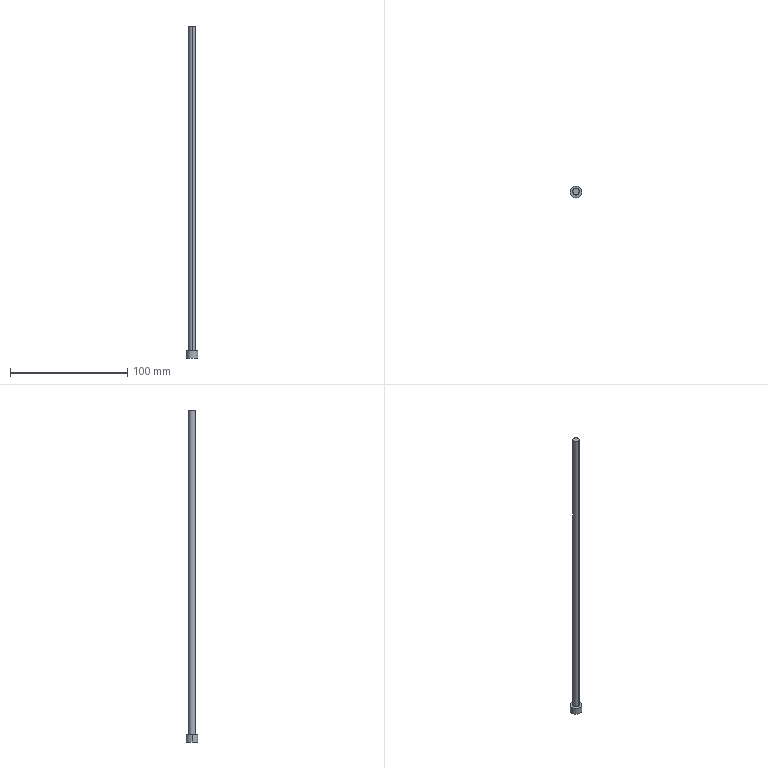Part | Creo | 1 solid | 7 faces | box 10 x 10 x 283.312 mm | volume 7060 mm3 | cylinder 4 | plane 3 | commonest cylinder face diameters 5.5 x2 10 x2
STEP:
#1=CARTESIAN_POINT('',(28.75,-153.,-12.688));
#2=VERTEX_POINT('',#1);
#3=CARTESIAN_POINT('',(26.,-150.25,-12.688));
#4=VERTEX_POINT('',#3);
#5=CARTESIAN_POINT('',(26.,-153.,-12.688));
#6=DIRECTION('',(0.,0.,1.));
#7=DIRECTION('',(1.,0.,0.));
#8=AXIS2_PLACEMENT_3D('',#5,#6,#7);
#9=CIRCLE('',#8,2.75);
#10=EDGE_CURVE('',#2,#4,#9,.T.);
#11=ORIENTED_EDGE('',*,*,#10,.F.);
#12=CARTESIAN_POINT('',(26.,-155.75,-12.688));
#13=VERTEX_POINT('',#12);
#14=CARTESIAN_POINT('',(26.,-153.,-12.688));
#15=DIRECTION('',(0.,0.,1.));
#16=DIRECTION('',(0.,-1.,0.));
#17=AXIS2_PLACEMENT_3D('',#14,#15,#16);
#18=CIRCLE('',#17,2.75);
#19=EDGE_CURVE('',#13,#2,#18,.T.);
#20=ORIENTED_EDGE('',*,*,#19,.F.);
#21=CARTESIAN_POINT('',(23.25,-153.,-12.688));
#22=VERTEX_POINT('',#21);
#23=CARTESIAN_POINT('',(26.,-153.,-12.688));
#24=DIRECTION('',(0.,0.,1.));
#25=DIRECTION('',(-1.,0.,0.));
#26=AXIS2_PLACEMENT_3D('',#23,#24,#25);
#27=CIRCLE('',#26,2.75);
#28=EDGE_CURVE('',#22,#13,#27,.T.);
#29=ORIENTED_EDGE('',*,*,#28,.F.);
#30=CARTESIAN_POINT('',(26.,-153.,-12.688));
#31=DIRECTION('',(0.,0.,1.));
#32=DIRECTION('',(0.,1.,0.));
#33=AXIS2_PLACEMENT_3D('',#30,#31,#32);
#34=CIRCLE('',#33,2.75);
#35=EDGE_CURVE('',#4,#22,#34,.T.);
#36=ORIENTED_EDGE('',*,*,#35,.F.);
#37=EDGE_LOOP('',(#11,#20,#29,#36));
#38=FACE_OUTER_BOUND('',#37,.F.);
#39=CARTESIAN_POINT('',(-2.3,-2.15,-12.688));
#40=DIRECTION('',(0.,0.,1.));
#41=DIRECTION('',(0.,-1.,0.));
#42=AXIS2_PLACEMENT_3D('',#39,#40,#41);
#43=PLANE('',#42);
#44=ADVANCED_FACE('',(#38),#43,.T.);
#45=CARTESIAN_POINT('',(26.,-150.25,-290.));
#46=VERTEX_POINT('',#45);
#47=CARTESIAN_POINT('',(28.75,-153.,-290.));
#48=VERTEX_POINT('',#47);
#49=CARTESIAN_POINT('',(26.,-153.,-290.));
#50=DIRECTION('',(0.,0.,-1.));
#51=DIRECTION('',(0.,1.,0.));
#52=AXIS2_PLACEMENT_3D('',#49,#50,#51);
#53=CIRCLE('',#52,2.75);
#54=EDGE_CURVE('',#46,#48,#53,.T.);
#55=ORIENTED_EDGE('',*,*,#54,.T.);
#56=CARTESIAN_POINT('',(26.,-155.75,-290.));
#57=VERTEX_POINT('',#56);
#58=CARTESIAN_POINT('',(26.,-153.,-290.));
#59=DIRECTION('',(0.,0.,-1.));
#60=DIRECTION('',(1.,0.,0.));
#61=AXIS2_PLACEMENT_3D('',#58,#59,#60);
#62=CIRCLE('',#61,2.75);
#63=EDGE_CURVE('',#48,#57,#62,.T.);
#64=ORIENTED_EDGE('',*,*,#63,.T.);
#65=CARTESIAN_POINT('',(26.,-155.75,-290.));
#66=DIRECTION('',(0.,0.,1.));
#67=VECTOR('',#66,277.312);
#68=LINE('',#65,#67);
#69=EDGE_CURVE('',#57,#13,#68,.T.);
#70=ORIENTED_EDGE('',*,*,#69,.T.);
#71=ORIENTED_EDGE('',*,*,#19,.T.);
#72=ORIENTED_EDGE('',*,*,#10,.T.);
#73=CARTESIAN_POINT('',(26.,-150.25,-290.));
#74=DIRECTION('',(0.,0.,1.));
#75=VECTOR('',#74,277.312);
#76=LINE('',#73,#75);
#77=EDGE_CURVE('',#46,#4,#76,.T.);
#78=ORIENTED_EDGE('',*,*,#77,.F.);
#79=EDGE_LOOP('',(#55,#64,#70,#71,#72,#78));
#80=FACE_OUTER_BOUND('',#79,.F.);
#81=CARTESIAN_POINT('',(26.,-153.,-351.57));
#82=DIRECTION('',(0.,0.,1.));
#83=DIRECTION('',(0.,-1.,0.));
#84=AXIS2_PLACEMENT_3D('',#81,#82,#83);
#85=CYLINDRICAL_SURFACE('',#84,2.75);
#86=ADVANCED_FACE('',(#80),#85,.T.);
#87=CARTESIAN_POINT('',(31.,-153.,-290.));
#88=VERTEX_POINT('',#87);
#89=CARTESIAN_POINT('',(21.,-153.,-290.));
#90=VERTEX_POINT('',#89);
#91=CARTESIAN_POINT('',(26.,-153.,-290.));
#92=DIRECTION('',(0.,0.,1.));
#93=DIRECTION('',(1.,0.,0.));
#94=AXIS2_PLACEMENT_3D('',#91,#92,#93);
#95=CIRCLE('',#94,5.);
#96=EDGE_CURVE('',#88,#90,#95,.T.);
#97=ORIENTED_EDGE('',*,*,#96,.F.);
#98=CARTESIAN_POINT('',(26.,-153.,-290.));
#99=DIRECTION('',(0.,0.,1.));
#100=DIRECTION('',(-1.,0.,0.));
#101=AXIS2_PLACEMENT_3D('',#98,#99,#100);
#102=CIRCLE('',#101,5.);
#103=EDGE_CURVE('',#90,#88,#102,.T.);
#104=ORIENTED_EDGE('',*,*,#103,.F.);
#105=EDGE_LOOP('',(#97,#104));
#106=FACE_OUTER_BOUND('',#105,.F.);
#107=ORIENTED_EDGE('',*,*,#63,.F.);
#108=ORIENTED_EDGE('',*,*,#54,.F.);
#109=CARTESIAN_POINT('',(23.25,-153.,-290.));
#110=VERTEX_POINT('',#109);
#111=CARTESIAN_POINT('',(26.,-153.,-290.));
#112=DIRECTION('',(0.,0.,-1.));
#113=DIRECTION('',(-1.,0.,0.));
#114=AXIS2_PLACEMENT_3D('',#111,#112,#113);
#115=CIRCLE('',#114,2.75);
#116=EDGE_CURVE('',#110,#46,#115,.T.);
#117=ORIENTED_EDGE('',*,*,#116,.F.);
#118=CARTESIAN_POINT('',(26.,-153.,-290.));
#119=DIRECTION('',(0.,0.,-1.));
#120=DIRECTION('',(0.,-1.,0.));
#121=AXIS2_PLACEMENT_3D('',#118,#119,#120);
#122=CIRCLE('',#121,2.75);
#123=EDGE_CURVE('',#57,#110,#122,.T.);
#124=ORIENTED_EDGE('',*,*,#123,.F.);
#125=EDGE_LOOP('',(#107,#108,#117,#124));
#126=FACE_BOUND('',#125,.F.);
#127=CARTESIAN_POINT('',(26.,-153.,-290.));
#128=DIRECTION('',(0.,0.,1.));
#129=DIRECTION('',(-1.,0.,0.));
#130=AXIS2_PLACEMENT_3D('',#127,#128,#129);
#131=PLANE('',#130);
#132=ADVANCED_FACE('',(#106,#126),#131,.T.);
#133=ORIENTED_EDGE('',*,*,#116,.T.);
#134=ORIENTED_EDGE('',*,*,#77,.T.);
#135=ORIENTED_EDGE('',*,*,#35,.T.);
#136=ORIENTED_EDGE('',*,*,#28,.T.);
#137=ORIENTED_EDGE('',*,*,#69,.F.);
#138=ORIENTED_EDGE('',*,*,#123,.T.);
#139=EDGE_LOOP('',(#133,#134,#135,#136,#137,#138));
#140=FACE_OUTER_BOUND('',#139,.F.);
#141=CARTESIAN_POINT('',(26.,-153.,-351.57));
#142=DIRECTION('',(0.,0.,1.));
#143=DIRECTION('',(0.,-1.,0.));
#144=AXIS2_PLACEMENT_3D('',#141,#142,#143);
#145=CYLINDRICAL_SURFACE('',#144,2.75);
#146=ADVANCED_FACE('',(#140),#145,.T.);
#147=ORIENTED_EDGE('',*,*,#96,.T.);
#148=CARTESIAN_POINT('',(21.,-153.,-296.));
#149=VERTEX_POINT('',#148);
#150=CARTESIAN_POINT('',(21.,-153.,-296.));
#151=DIRECTION('',(0.,0.,1.));
#152=VECTOR('',#151,6.);
#153=LINE('',#150,#152);
#154=EDGE_CURVE('',#149,#90,#153,.T.);
#155=ORIENTED_EDGE('',*,*,#154,.F.);
#156=CARTESIAN_POINT('',(31.,-153.,-296.));
#157=VERTEX_POINT('',#156);
#158=CARTESIAN_POINT('',(26.,-153.,-296.));
#159=DIRECTION('',(0.,0.,-1.));
#160=DIRECTION('',(-1.,0.,0.));
#161=AXIS2_PLACEMENT_3D('',#158,#159,#160);
#162=CIRCLE('',#161,5.);
#163=EDGE_CURVE('',#149,#157,#162,.T.);
#164=ORIENTED_EDGE('',*,*,#163,.T.);
#165=CARTESIAN_POINT('',(31.,-153.,-296.));
#166=DIRECTION('',(0.,0.,1.));
#167=VECTOR('',#166,6.);
#168=LINE('',#165,#167);
#169=EDGE_CURVE('',#157,#88,#168,.T.);
#170=ORIENTED_EDGE('',*,*,#169,.T.);
#171=EDGE_LOOP('',(#147,#155,#164,#170));
#172=FACE_OUTER_BOUND('',#171,.F.);
#173=CARTESIAN_POINT('',(26.,-153.,-296.));
#174=DIRECTION('',(0.,0.,1.));
#175=DIRECTION('',(-1.,0.,0.));
#176=AXIS2_PLACEMENT_3D('',#173,#174,#175);
#177=CYLINDRICAL_SURFACE('',#176,5.);
#178=ADVANCED_FACE('',(#172),#177,.T.);
#179=ORIENTED_EDGE('',*,*,#103,.T.);
#180=ORIENTED_EDGE('',*,*,#169,.F.);
#181=CARTESIAN_POINT('',(26.,-153.,-296.));
#182=DIRECTION('',(0.,0.,-1.));
#183=DIRECTION('',(1.,0.,0.));
#184=AXIS2_PLACEMENT_3D('',#181,#182,#183);
#185=CIRCLE('',#184,5.);
#186=EDGE_CURVE('',#157,#149,#185,.T.);
#187=ORIENTED_EDGE('',*,*,#186,.T.);
#188=ORIENTED_EDGE('',*,*,#154,.T.);
#189=EDGE_LOOP('',(#179,#180,#187,#188));
#190=FACE_OUTER_BOUND('',#189,.F.);
#191=CARTESIAN_POINT('',(26.,-153.,-296.));
#192=DIRECTION('',(0.,0.,1.));
#193=DIRECTION('',(-1.,0.,0.));
#194=AXIS2_PLACEMENT_3D('',#191,#192,#193);
#195=CYLINDRICAL_SURFACE('',#194,5.);
#196=ADVANCED_FACE('',(#190),#195,.T.);
#197=ORIENTED_EDGE('',*,*,#186,.F.);
#198=ORIENTED_EDGE('',*,*,#163,.F.);
#199=EDGE_LOOP('',(#197,#198));
#200=FACE_OUTER_BOUND('',#199,.F.);
#201=CARTESIAN_POINT('',(7.7,-2.155,-296.));
#202=DIRECTION('',(0.,0.,1.));
#203=DIRECTION('',(0.,1.,0.));
#204=AXIS2_PLACEMENT_3D('',#201,#202,#203);
#205=PLANE('',#204);
#206=ADVANCED_FACE('',(#200),#205,.F.);
#207=CLOSED_SHELL('',(#44,#86,#132,#146,#178,#196,#206));
#208=MANIFOLD_SOLID_BREP('',#207);
#209=(LENGTH_UNIT()NAMED_UNIT(*)SI_UNIT(.MILLI.,.METRE.));
#210=UNCERTAINTY_MEASURE_WITH_UNIT(LENGTH_MEASURE(0.02837),#209,'','');
#211=(NAMED_UNIT(*)PLANE_ANGLE_UNIT()SI_UNIT($,.RADIAN.));
#212=PLANE_ANGLE_MEASURE_WITH_UNIT(PLANE_ANGLE_MEASURE(0.01745),#211);
#213=(CONVERSION_BASED_UNIT('DEGREE',#212)NAMED_UNIT(*)PLANE_ANGLE_UNIT());
#214=(NAMED_UNIT(*)SI_UNIT($,.STERADIAN.)SOLID_ANGLE_UNIT());
#215=(GEOMETRIC_REPRESENTATION_CONTEXT(3)GLOBAL_UNCERTAINTY_ASSIGNED_CONTEXT((#210))GLOBAL_UNIT_ASSIGNED_CONTEXT((#209,#213,#214))REPRESENTATION_CONTEXT('',''));
#216=ADVANCED_BREP_SHAPE_REPRESENTATION('',(#208),#215);